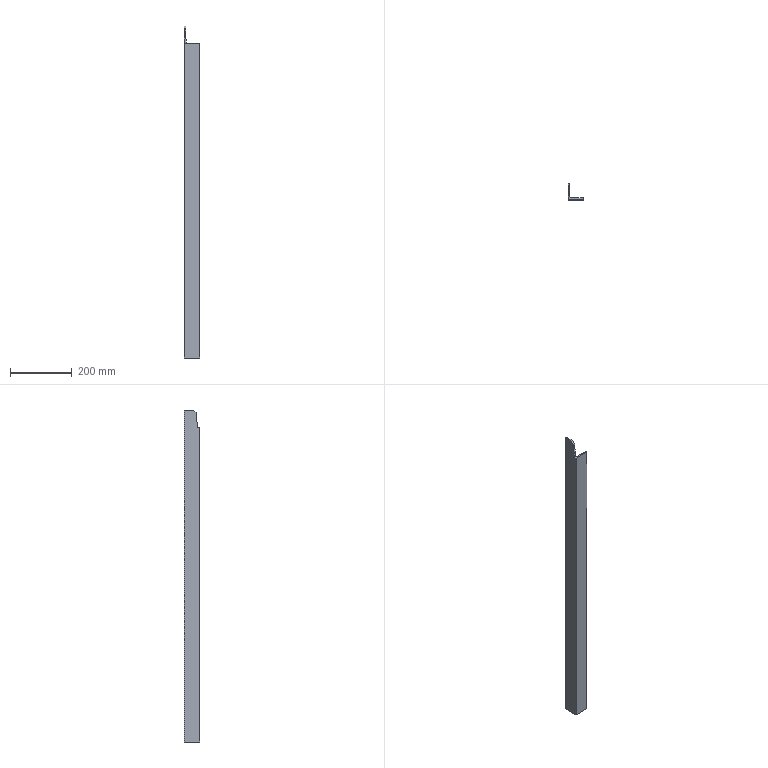Part | SolidWorks | 1 solid | 15 faces | box 50 x 50 x 1074 mm | volume 499534 mm3 | plane 12 | cylinder 3 | commonest cylinder face diameters 3.333 x2 11 x1
STEP:
#1=CARTESIAN_POINT('',(0.,0.,-1073.5));
#2=VERTEX_POINT('',#1);
#3=CARTESIAN_POINT('',(0.,0.,-56.5));
#4=VERTEX_POINT('',#3);
#5=CARTESIAN_POINT('',(0.,0.,-1073.5));
#6=DIRECTION('',(0.,0.,1.));
#7=VECTOR('',#6,1000.);
#8=LINE('',#5,#7);
#9=EDGE_CURVE('',#2,#4,#8,.T.);
#10=ORIENTED_EDGE('',*,*,#9,.T.);
#11=CARTESIAN_POINT('',(0.,7.501,-56.5));
#12=VERTEX_POINT('',#11);
#13=CARTESIAN_POINT('',(0.,0.,-56.5));
#14=DIRECTION('',(0.,-1.,0.));
#15=VECTOR('',#14,1000.);
#16=LINE('',#13,#15);
#17=EDGE_CURVE('',#12,#4,#16,.T.);
#18=ORIENTED_EDGE('',*,*,#17,.F.);
#19=CARTESIAN_POINT('',(0.,7.501,-52.023));
#20=VERTEX_POINT('',#19);
#21=CARTESIAN_POINT('',(0.,7.501,-56.5));
#22=DIRECTION('',(0.,0.,-1.));
#23=VECTOR('',#22,1000.);
#24=LINE('',#21,#23);
#25=EDGE_CURVE('',#20,#12,#24,.T.);
#26=ORIENTED_EDGE('',*,*,#25,.F.);
#27=CARTESIAN_POINT('',(0.,12.028,-8.955));
#28=VERTEX_POINT('',#27);
#29=CARTESIAN_POINT('',(0.,7.501,-52.023));
#30=DIRECTION('',(0.,-0.1045,-0.9945));
#31=VECTOR('',#30,1000.);
#32=LINE('',#29,#31);
#33=EDGE_CURVE('',#28,#20,#32,.T.);
#34=ORIENTED_EDGE('',*,*,#33,.F.);
#35=CARTESIAN_POINT('',(0.,21.973,0.));
#36=VERTEX_POINT('',#35);
#37=CARTESIAN_POINT('',(0.,12.028,-8.955));
#38=DIRECTION('',(0.,-0.7431,-0.6691));
#39=VECTOR('',#38,1000.);
#40=LINE('',#37,#39);
#41=EDGE_CURVE('',#36,#28,#40,.T.);
#42=ORIENTED_EDGE('',*,*,#41,.F.);
#43=CARTESIAN_POINT('',(0.,50.,0.));
#44=VERTEX_POINT('',#43);
#45=CARTESIAN_POINT('',(0.,50.,0.));
#46=DIRECTION('',(0.,1.,0.));
#47=VECTOR('',#46,1000.);
#48=LINE('',#45,#47);
#49=EDGE_CURVE('',#36,#44,#48,.T.);
#50=ORIENTED_EDGE('',*,*,#49,.T.);
#51=CARTESIAN_POINT('',(0.,50.,-1073.5));
#52=VERTEX_POINT('',#51);
#53=CARTESIAN_POINT('',(0.,50.,-1073.5));
#54=DIRECTION('',(0.,0.,1.));
#55=VECTOR('',#54,1000.);
#56=LINE('',#53,#55);
#57=EDGE_CURVE('',#52,#44,#56,.T.);
#58=ORIENTED_EDGE('',*,*,#57,.F.);
#59=CARTESIAN_POINT('',(0.,50.,-1073.5));
#60=DIRECTION('',(0.,1.,0.));
#61=VECTOR('',#60,1000.);
#62=LINE('',#59,#61);
#63=EDGE_CURVE('',#2,#52,#62,.T.);
#64=ORIENTED_EDGE('',*,*,#63,.F.);
#65=EDGE_LOOP('',(#10,#18,#26,#34,#42,#50,#58,#64));
#66=FACE_OUTER_BOUND('',#65,.T.);
#67=CARTESIAN_POINT('',(0.,50.,-1073.5));
#68=DIRECTION('',(1.,0.,0.));
#69=DIRECTION('',(0.,0.,-1.));
#70=AXIS2_PLACEMENT_3D('',#67,#68,#69);
#71=PLANE('',#70);
#72=ADVANCED_FACE('',(#66),#71,.F.);
#73=CARTESIAN_POINT('',(3.333,50.,0.));
#74=VERTEX_POINT('',#73);
#75=CARTESIAN_POINT('',(0.,50.,0.));
#76=DIRECTION('',(1.,0.,0.));
#77=VECTOR('',#76,1000.);
#78=LINE('',#75,#77);
#79=EDGE_CURVE('',#44,#74,#78,.T.);
#80=ORIENTED_EDGE('',*,*,#79,.T.);
#81=CARTESIAN_POINT('',(3.333,50.,-1073.5));
#82=VERTEX_POINT('',#81);
#83=CARTESIAN_POINT('',(3.333,50.,-1073.5));
#84=DIRECTION('',(0.,0.,1.));
#85=VECTOR('',#84,1000.);
#86=LINE('',#83,#85);
#87=EDGE_CURVE('',#82,#74,#86,.T.);
#88=ORIENTED_EDGE('',*,*,#87,.F.);
#89=CARTESIAN_POINT('',(0.,50.,-1073.5));
#90=DIRECTION('',(1.,0.,0.));
#91=VECTOR('',#90,1000.);
#92=LINE('',#89,#91);
#93=EDGE_CURVE('',#52,#82,#92,.T.);
#94=ORIENTED_EDGE('',*,*,#93,.F.);
#95=ORIENTED_EDGE('',*,*,#57,.T.);
#96=EDGE_LOOP('',(#80,#88,#94,#95));
#97=FACE_OUTER_BOUND('',#96,.T.);
#98=CARTESIAN_POINT('',(0.,50.,-1073.5));
#99=DIRECTION('',(0.,-1.,0.));
#100=DIRECTION('',(0.,0.,-1.));
#101=AXIS2_PLACEMENT_3D('',#98,#99,#100);
#102=PLANE('',#101);
#103=ADVANCED_FACE('',(#97),#102,.F.);
#104=CARTESIAN_POINT('',(5.,48.333,0.));
#105=VERTEX_POINT('',#104);
#106=CARTESIAN_POINT('',(3.333,48.333,0.));
#107=DIRECTION('',(0.,0.,-1.));
#108=DIRECTION('',(-1.,0.,0.));
#109=AXIS2_PLACEMENT_3D('',#106,#107,#108);
#110=CIRCLE('',#109,1.667);
#111=EDGE_CURVE('',#74,#105,#110,.T.);
#112=ORIENTED_EDGE('',*,*,#111,.T.);
#113=CARTESIAN_POINT('',(5.,48.333,-1073.5));
#114=VERTEX_POINT('',#113);
#115=CARTESIAN_POINT('',(5.,48.333,-1073.5));
#116=DIRECTION('',(0.,0.,1.));
#117=VECTOR('',#116,1000.);
#118=LINE('',#115,#117);
#119=EDGE_CURVE('',#114,#105,#118,.T.);
#120=ORIENTED_EDGE('',*,*,#119,.F.);
#121=CARTESIAN_POINT('',(3.333,48.333,-1073.5));
#122=DIRECTION('',(0.,0.,-1.));
#123=DIRECTION('',(-1.,0.,0.));
#124=AXIS2_PLACEMENT_3D('',#121,#122,#123);
#125=CIRCLE('',#124,1.667);
#126=EDGE_CURVE('',#82,#114,#125,.T.);
#127=ORIENTED_EDGE('',*,*,#126,.F.);
#128=ORIENTED_EDGE('',*,*,#87,.T.);
#129=EDGE_LOOP('',(#112,#120,#127,#128));
#130=FACE_OUTER_BOUND('',#129,.T.);
#131=CARTESIAN_POINT('',(3.333,48.333,-1073.5));
#132=DIRECTION('',(0.,0.,1.));
#133=DIRECTION('',(1.,0.,0.));
#134=AXIS2_PLACEMENT_3D('',#131,#132,#133);
#135=CYLINDRICAL_SURFACE('',#134,1.667);
#136=ADVANCED_FACE('',(#130),#135,.T.);
#137=CARTESIAN_POINT('',(5.,21.973,0.));
#138=VERTEX_POINT('',#137);
#139=CARTESIAN_POINT('',(5.,10.5,0.));
#140=DIRECTION('',(0.,-1.,0.));
#141=VECTOR('',#140,1000.);
#142=LINE('',#139,#141);
#143=EDGE_CURVE('',#105,#138,#142,.T.);
#144=ORIENTED_EDGE('',*,*,#143,.T.);
#145=CARTESIAN_POINT('',(5.,12.028,-8.955));
#146=VERTEX_POINT('',#145);
#147=CARTESIAN_POINT('',(5.,12.028,-8.955));
#148=DIRECTION('',(0.,0.7431,0.6691));
#149=VECTOR('',#148,1000.);
#150=LINE('',#147,#149);
#151=EDGE_CURVE('',#146,#138,#150,.T.);
#152=ORIENTED_EDGE('',*,*,#151,.F.);
#153=CARTESIAN_POINT('',(5.,10.5,-23.493));
#154=VERTEX_POINT('',#153);
#155=CARTESIAN_POINT('',(5.,7.501,-52.023));
#156=DIRECTION('',(0.,0.1045,0.9945));
#157=VECTOR('',#156,1000.);
#158=LINE('',#155,#157);
#159=EDGE_CURVE('',#154,#146,#158,.T.);
#160=ORIENTED_EDGE('',*,*,#159,.F.);
#161=CARTESIAN_POINT('',(5.,10.5,-1073.5));
#162=VERTEX_POINT('',#161);
#163=CARTESIAN_POINT('',(5.,10.5,-1073.5));
#164=DIRECTION('',(0.,0.,1.));
#165=VECTOR('',#164,1000.);
#166=LINE('',#163,#165);
#167=EDGE_CURVE('',#162,#154,#166,.T.);
#168=ORIENTED_EDGE('',*,*,#167,.F.);
#169=CARTESIAN_POINT('',(5.,10.5,-1073.5));
#170=DIRECTION('',(0.,-1.,0.));
#171=VECTOR('',#170,1000.);
#172=LINE('',#169,#171);
#173=EDGE_CURVE('',#114,#162,#172,.T.);
#174=ORIENTED_EDGE('',*,*,#173,.F.);
#175=ORIENTED_EDGE('',*,*,#119,.T.);
#176=EDGE_LOOP('',(#144,#152,#160,#168,#174,#175));
#177=FACE_OUTER_BOUND('',#176,.T.);
#178=CARTESIAN_POINT('',(5.,10.5,-1073.5));
#179=DIRECTION('',(-1.,0.,0.));
#180=DIRECTION('',(0.,-1.,0.));
#181=AXIS2_PLACEMENT_3D('',#178,#179,#180);
#182=PLANE('',#181);
#183=ADVANCED_FACE('',(#177),#182,.F.);
#184=CARTESIAN_POINT('',(5.889,7.501,-56.5));
#185=VERTEX_POINT('',#184);
#186=CARTESIAN_POINT('',(5.889,7.501,-52.023));
#187=VERTEX_POINT('',#186);
#188=CARTESIAN_POINT('',(5.889,7.501,-1073.5));
#189=DIRECTION('',(0.,0.,1.));
#190=VECTOR('',#189,1000.);
#191=LINE('',#188,#190);
#192=EDGE_CURVE('',#185,#187,#191,.T.);
#193=ORIENTED_EDGE('',*,*,#192,.F.);
#194=CARTESIAN_POINT('',(10.5,5.,-56.5));
#195=VERTEX_POINT('',#194);
#196=CARTESIAN_POINT('',(10.5,10.5,-56.5));
#197=DIRECTION('',(0.,0.,-1.));
#198=DIRECTION('',(0.,1.,0.));
#199=AXIS2_PLACEMENT_3D('',#196,#197,#198);
#200=CIRCLE('',#199,5.5);
#201=EDGE_CURVE('',#195,#185,#200,.T.);
#202=ORIENTED_EDGE('',*,*,#201,.F.);
#203=CARTESIAN_POINT('',(10.5,5.,-1073.5));
#204=VERTEX_POINT('',#203);
#205=CARTESIAN_POINT('',(10.5,5.,-1073.5));
#206=DIRECTION('',(0.,0.,1.));
#207=VECTOR('',#206,1000.);
#208=LINE('',#205,#207);
#209=EDGE_CURVE('',#204,#195,#208,.T.);
#210=ORIENTED_EDGE('',*,*,#209,.F.);
#211=CARTESIAN_POINT('',(10.5,10.5,-1073.5));
#212=DIRECTION('',(0.,0.,1.));
#213=DIRECTION('',(1.,0.,0.));
#214=AXIS2_PLACEMENT_3D('',#211,#212,#213);
#215=CIRCLE('',#214,5.5);
#216=EDGE_CURVE('',#162,#204,#215,.T.);
#217=ORIENTED_EDGE('',*,*,#216,.F.);
#218=ORIENTED_EDGE('',*,*,#167,.T.);
#219=CARTESIAN_POINT('',(5.889,7.501,-52.023));
#220=CARTESIAN_POINT('',(5.305,8.4,-43.472));
#221=CARTESIAN_POINT('',(5.,9.428,-33.693));
#222=CARTESIAN_POINT('',(5.,10.5,-23.493));
#223=(BOUNDED_CURVE()B_SPLINE_CURVE(3,(#219,#220,#221,#222),.UNSPECIFIED.,.F.,.T.)B_SPLINE_CURVE_WITH_KNOTS((4,4),(4.136,4.712),.UNSPECIFIED.)CURVE()GEOMETRIC_REPRESENTATION_ITEM()RATIONAL_B_SPLINE_CURVE((1.,0.9725,0.9725,1.))REPRESENTATION_ITEM(''));
#224=EDGE_CURVE('',#187,#154,#223,.T.);
#225=ORIENTED_EDGE('',*,*,#224,.F.);
#226=EDGE_LOOP('',(#193,#202,#210,#217,#218,#225));
#227=FACE_OUTER_BOUND('',#226,.T.);
#228=CARTESIAN_POINT('',(10.5,10.5,-1073.5));
#229=DIRECTION('',(0.,0.,1.));
#230=DIRECTION('',(1.,0.,0.));
#231=AXIS2_PLACEMENT_3D('',#228,#229,#230);
#232=CYLINDRICAL_SURFACE('',#231,5.5);
#233=ADVANCED_FACE('',(#227),#232,.F.);
#234=ORIENTED_EDGE('',*,*,#209,.T.);
#235=CARTESIAN_POINT('',(48.333,5.,-56.5));
#236=VERTEX_POINT('',#235);
#237=CARTESIAN_POINT('',(50.001,5.,-56.5));
#238=DIRECTION('',(-1.,0.,0.));
#239=VECTOR('',#238,1000.);
#240=LINE('',#237,#239);
#241=EDGE_CURVE('',#236,#195,#240,.T.);
#242=ORIENTED_EDGE('',*,*,#241,.F.);
#243=CARTESIAN_POINT('',(48.333,5.,-1073.5));
#244=VERTEX_POINT('',#243);
#245=CARTESIAN_POINT('',(48.333,5.,-1073.5));
#246=DIRECTION('',(0.,0.,1.));
#247=VECTOR('',#246,1000.);
#248=LINE('',#245,#247);
#249=EDGE_CURVE('',#244,#236,#248,.T.);
#250=ORIENTED_EDGE('',*,*,#249,.F.);
#251=CARTESIAN_POINT('',(48.333,5.,-1073.5));
#252=DIRECTION('',(1.,0.,0.));
#253=VECTOR('',#252,1000.);
#254=LINE('',#251,#253);
#255=EDGE_CURVE('',#204,#244,#254,.T.);
#256=ORIENTED_EDGE('',*,*,#255,.F.);
#257=EDGE_LOOP('',(#234,#242,#250,#256));
#258=FACE_OUTER_BOUND('',#257,.T.);
#259=CARTESIAN_POINT('',(48.333,5.,-1073.5));
#260=DIRECTION('',(0.,-1.,0.));
#261=DIRECTION('',(1.,0.,0.));
#262=AXIS2_PLACEMENT_3D('',#259,#260,#261);
#263=PLANE('',#262);
#264=ADVANCED_FACE('',(#258),#263,.F.);
#265=ORIENTED_EDGE('',*,*,#249,.T.);
#266=CARTESIAN_POINT('',(50.,3.333,-56.5));
#267=VERTEX_POINT('',#266);
#268=CARTESIAN_POINT('',(48.333,3.333,-56.5));
#269=DIRECTION('',(0.,0.,1.));
#270=DIRECTION('',(0.,1.,0.));
#271=AXIS2_PLACEMENT_3D('',#268,#269,#270);
#272=CIRCLE('',#271,1.667);
#273=EDGE_CURVE('',#267,#236,#272,.T.);
#274=ORIENTED_EDGE('',*,*,#273,.F.);
#275=CARTESIAN_POINT('',(50.,3.333,-1073.5));
#276=VERTEX_POINT('',#275);
#277=CARTESIAN_POINT('',(50.,3.333,-1073.5));
#278=DIRECTION('',(0.,0.,1.));
#279=VECTOR('',#278,1000.);
#280=LINE('',#277,#279);
#281=EDGE_CURVE('',#276,#267,#280,.T.);
#282=ORIENTED_EDGE('',*,*,#281,.F.);
#283=CARTESIAN_POINT('',(48.333,3.333,-1073.5));
#284=DIRECTION('',(0.,0.,-1.));
#285=DIRECTION('',(1.,0.,0.));
#286=AXIS2_PLACEMENT_3D('',#283,#284,#285);
#287=CIRCLE('',#286,1.667);
#288=EDGE_CURVE('',#244,#276,#287,.T.);
#289=ORIENTED_EDGE('',*,*,#288,.F.);
#290=EDGE_LOOP('',(#265,#274,#282,#289));
#291=FACE_OUTER_BOUND('',#290,.T.);
#292=CARTESIAN_POINT('',(48.333,3.333,-1073.5));
#293=DIRECTION('',(0.,0.,1.));
#294=DIRECTION('',(1.,0.,0.));
#295=AXIS2_PLACEMENT_3D('',#292,#293,#294);
#296=CYLINDRICAL_SURFACE('',#295,1.667);
#297=ADVANCED_FACE('',(#291),#296,.T.);
#298=ORIENTED_EDGE('',*,*,#281,.T.);
#299=CARTESIAN_POINT('',(50.,0.,-56.5));
#300=VERTEX_POINT('',#299);
#301=CARTESIAN_POINT('',(50.,0.,-56.5));
#302=DIRECTION('',(0.,1.,0.));
#303=VECTOR('',#302,1000.);
#304=LINE('',#301,#303);
#305=EDGE_CURVE('',#300,#267,#304,.T.);
#306=ORIENTED_EDGE('',*,*,#305,.F.);
#307=CARTESIAN_POINT('',(50.,0.,-1073.5));
#308=VERTEX_POINT('',#307);
#309=CARTESIAN_POINT('',(50.,0.,-1073.5));
#310=DIRECTION('',(0.,0.,1.));
#311=VECTOR('',#310,1000.);
#312=LINE('',#309,#311);
#313=EDGE_CURVE('',#308,#300,#312,.T.);
#314=ORIENTED_EDGE('',*,*,#313,.F.);
#315=CARTESIAN_POINT('',(50.,0.,-1073.5));
#316=DIRECTION('',(0.,-1.,0.));
#317=VECTOR('',#316,1000.);
#318=LINE('',#315,#317);
#319=EDGE_CURVE('',#276,#308,#318,.T.);
#320=ORIENTED_EDGE('',*,*,#319,.F.);
#321=EDGE_LOOP('',(#298,#306,#314,#320));
#322=FACE_OUTER_BOUND('',#321,.T.);
#323=CARTESIAN_POINT('',(50.,0.,-1073.5));
#324=DIRECTION('',(-1.,0.,0.));
#325=DIRECTION('',(0.,-1.,0.));
#326=AXIS2_PLACEMENT_3D('',#323,#324,#325);
#327=PLANE('',#326);
#328=ADVANCED_FACE('',(#322),#327,.F.);
#329=ORIENTED_EDGE('',*,*,#313,.T.);
#330=CARTESIAN_POINT('',(50.001,0.,-56.5));
#331=DIRECTION('',(1.,0.,0.));
#332=VECTOR('',#331,1000.);
#333=LINE('',#330,#332);
#334=EDGE_CURVE('',#4,#300,#333,.T.);
#335=ORIENTED_EDGE('',*,*,#334,.F.);
#336=ORIENTED_EDGE('',*,*,#9,.F.);
#337=CARTESIAN_POINT('',(0.,0.,-1073.5));
#338=DIRECTION('',(-1.,0.,0.));
#339=VECTOR('',#338,1000.);
#340=LINE('',#337,#339);
#341=EDGE_CURVE('',#308,#2,#340,.T.);
#342=ORIENTED_EDGE('',*,*,#341,.F.);
#343=EDGE_LOOP('',(#329,#335,#336,#342));
#344=FACE_OUTER_BOUND('',#343,.T.);
#345=CARTESIAN_POINT('',(0.,0.,-1073.5));
#346=DIRECTION('',(0.,1.,0.));
#347=DIRECTION('',(0.,0.,1.));
#348=AXIS2_PLACEMENT_3D('',#345,#346,#347);
#349=PLANE('',#348);
#350=ADVANCED_FACE('',(#344),#349,.F.);
#351=ORIENTED_EDGE('',*,*,#63,.T.);
#352=ORIENTED_EDGE('',*,*,#93,.T.);
#353=ORIENTED_EDGE('',*,*,#126,.T.);
#354=ORIENTED_EDGE('',*,*,#173,.T.);
#355=ORIENTED_EDGE('',*,*,#216,.T.);
#356=ORIENTED_EDGE('',*,*,#255,.T.);
#357=ORIENTED_EDGE('',*,*,#288,.T.);
#358=ORIENTED_EDGE('',*,*,#319,.T.);
#359=ORIENTED_EDGE('',*,*,#341,.T.);
#360=EDGE_LOOP('',(#351,#352,#353,#354,#355,#356,#357,#358,#359));
#361=FACE_OUTER_BOUND('',#360,.T.);
#362=CARTESIAN_POINT('',(48.333,3.333,-1073.5));
#363=DIRECTION('',(0.,0.,1.));
#364=DIRECTION('',(1.,0.,0.));
#365=AXIS2_PLACEMENT_3D('',#362,#363,#364);
#366=PLANE('',#365);
#367=ADVANCED_FACE('',(#361),#366,.F.);
#368=CARTESIAN_POINT('',(50.001,21.973,0.));
#369=DIRECTION('',(1.,0.,0.));
#370=VECTOR('',#369,1000.);
#371=LINE('',#368,#370);
#372=EDGE_CURVE('',#36,#138,#371,.T.);
#373=ORIENTED_EDGE('',*,*,#372,.T.);
#374=ORIENTED_EDGE('',*,*,#143,.F.);
#375=ORIENTED_EDGE('',*,*,#111,.F.);
#376=ORIENTED_EDGE('',*,*,#79,.F.);
#377=ORIENTED_EDGE('',*,*,#49,.F.);
#378=EDGE_LOOP('',(#373,#374,#375,#376,#377));
#379=FACE_OUTER_BOUND('',#378,.T.);
#380=CARTESIAN_POINT('',(48.333,3.333,0.));
#381=DIRECTION('',(0.,0.,1.));
#382=DIRECTION('',(1.,0.,0.));
#383=AXIS2_PLACEMENT_3D('',#380,#381,#382);
#384=PLANE('',#383);
#385=ADVANCED_FACE('',(#379),#384,.T.);
#386=ORIENTED_EDGE('',*,*,#201,.T.);
#387=CARTESIAN_POINT('',(50.001,7.501,-56.5));
#388=DIRECTION('',(-1.,0.,0.));
#389=VECTOR('',#388,1000.);
#390=LINE('',#387,#389);
#391=EDGE_CURVE('',#185,#12,#390,.T.);
#392=ORIENTED_EDGE('',*,*,#391,.T.);
#393=ORIENTED_EDGE('',*,*,#17,.T.);
#394=ORIENTED_EDGE('',*,*,#334,.T.);
#395=ORIENTED_EDGE('',*,*,#305,.T.);
#396=ORIENTED_EDGE('',*,*,#273,.T.);
#397=ORIENTED_EDGE('',*,*,#241,.T.);
#398=EDGE_LOOP('',(#386,#392,#393,#394,#395,#396,#397));
#399=FACE_OUTER_BOUND('',#398,.T.);
#400=CARTESIAN_POINT('',(50.001,0.,-56.5));
#401=DIRECTION('',(0.,0.,-1.));
#402=DIRECTION('',(0.,1.,0.));
#403=AXIS2_PLACEMENT_3D('',#400,#401,#402);
#404=PLANE('',#403);
#405=ADVANCED_FACE('',(#399),#404,.F.);
#406=ORIENTED_EDGE('',*,*,#192,.T.);
#407=CARTESIAN_POINT('',(50.001,7.501,-52.023));
#408=DIRECTION('',(-1.,0.,0.));
#409=VECTOR('',#408,1000.);
#410=LINE('',#407,#409);
#411=EDGE_CURVE('',#187,#20,#410,.T.);
#412=ORIENTED_EDGE('',*,*,#411,.T.);
#413=ORIENTED_EDGE('',*,*,#25,.T.);
#414=ORIENTED_EDGE('',*,*,#391,.F.);
#415=EDGE_LOOP('',(#406,#412,#413,#414));
#416=FACE_OUTER_BOUND('',#415,.T.);
#417=CARTESIAN_POINT('',(50.001,7.501,-56.5));
#418=DIRECTION('',(0.,1.,0.));
#419=DIRECTION('',(0.,0.,1.));
#420=AXIS2_PLACEMENT_3D('',#417,#418,#419);
#421=PLANE('',#420);
#422=ADVANCED_FACE('',(#416),#421,.F.);
#423=ORIENTED_EDGE('',*,*,#151,.T.);
#424=ORIENTED_EDGE('',*,*,#372,.F.);
#425=ORIENTED_EDGE('',*,*,#41,.T.);
#426=CARTESIAN_POINT('',(50.001,12.028,-8.955));
#427=DIRECTION('',(-1.,0.,0.));
#428=VECTOR('',#427,1000.);
#429=LINE('',#426,#428);
#430=EDGE_CURVE('',#146,#28,#429,.T.);
#431=ORIENTED_EDGE('',*,*,#430,.F.);
#432=EDGE_LOOP('',(#423,#424,#425,#431));
#433=FACE_OUTER_BOUND('',#432,.T.);
#434=CARTESIAN_POINT('',(50.001,12.028,-8.955));
#435=DIRECTION('',(0.,0.6691,-0.7431));
#436=DIRECTION('',(0.,0.7431,0.6691));
#437=AXIS2_PLACEMENT_3D('',#434,#435,#436);
#438=PLANE('',#437);
#439=ADVANCED_FACE('',(#433),#438,.F.);
#440=ORIENTED_EDGE('',*,*,#159,.T.);
#441=ORIENTED_EDGE('',*,*,#430,.T.);
#442=ORIENTED_EDGE('',*,*,#33,.T.);
#443=ORIENTED_EDGE('',*,*,#411,.F.);
#444=ORIENTED_EDGE('',*,*,#224,.T.);
#445=EDGE_LOOP('',(#440,#441,#442,#443,#444));
#446=FACE_OUTER_BOUND('',#445,.T.);
#447=CARTESIAN_POINT('',(50.001,7.501,-52.023));
#448=DIRECTION('',(0.,0.9945,-0.1045));
#449=DIRECTION('',(0.,0.1045,0.9945));
#450=AXIS2_PLACEMENT_3D('',#447,#448,#449);
#451=PLANE('',#450);
#452=ADVANCED_FACE('',(#446),#451,.F.);
#453=CLOSED_SHELL('',(#72,#103,#136,#183,#233,#264,#297,#328,#350,#367,#385,#405,#422,#439,#452));
#454=MANIFOLD_SOLID_BREP('',#453);
#455=CARTESIAN_POINT('',(0.,0.,0.));
#456=DIRECTION('',(0.,0.,1.));
#457=DIRECTION('',(1.,0.,0.));
#458=AXIS2_PLACEMENT_3D('',#455,#456,#457);
#459=(LENGTH_UNIT()NAMED_UNIT(*)SI_UNIT(.MILLI.,.METRE.));
#460=UNCERTAINTY_MEASURE_WITH_UNIT(LENGTH_MEASURE(0.00001),#459,'','');
#461=(NAMED_UNIT(*)PLANE_ANGLE_UNIT()SI_UNIT($,.RADIAN.));
#462=(NAMED_UNIT(*)SI_UNIT($,.STERADIAN.)SOLID_ANGLE_UNIT());
#463=(GEOMETRIC_REPRESENTATION_CONTEXT(3)GLOBAL_UNCERTAINTY_ASSIGNED_CONTEXT((#460))GLOBAL_UNIT_ASSIGNED_CONTEXT((#459,#461,#462))REPRESENTATION_CONTEXT('',''));
#464=ADVANCED_BREP_SHAPE_REPRESENTATION('',(#454,#458),#463);